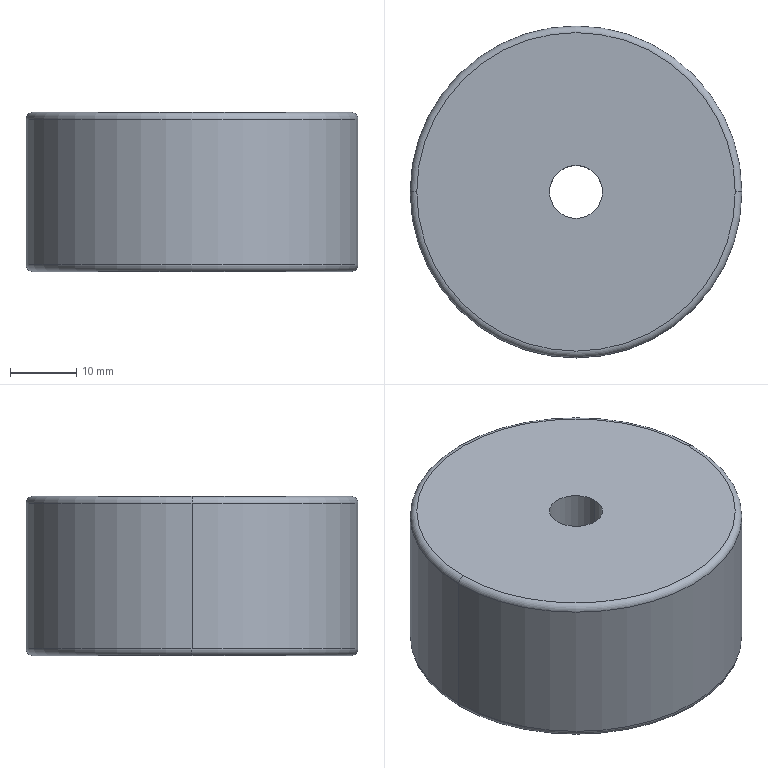Part | SolidWorks | features Extrusion 1, Fillet 1, ICE 1 | 1 solid | 10 faces | box 50 x 50 x 24 mm | volume 45851 mm3 | torus 4 | cylinder 4 | plane 2 | commonest cylinder face diameters 8 x2 50 x2
STEP:
#1=CARTESIAN_POINT('',(-25.,0.,23.));
#2=VERTEX_POINT('',#1);
#3=CARTESIAN_POINT('',(25.,0.,23.));
#4=VERTEX_POINT('',#3);
#5=CARTESIAN_POINT('',(0.,0.,23.));
#6=DIRECTION('',(0.,0.,-1.));
#7=DIRECTION('',(1.,0.,0.));
#8=AXIS2_PLACEMENT_3D('',#5,#6,#7);
#9=CIRCLE('',#8,25.);
#10=EDGE_CURVE('',#2,#4,#9,.T.);
#11=ORIENTED_EDGE('',*,*,#10,.F.);
#12=CARTESIAN_POINT('',(-24.,0.,24.));
#13=VERTEX_POINT('',#12);
#14=CARTESIAN_POINT('',(-24.,0.,23.));
#15=DIRECTION('',(0.,1.,0.));
#16=DIRECTION('',(-1.,0.,0.));
#17=AXIS2_PLACEMENT_3D('',#14,#15,#16);
#18=CIRCLE('',#17,1.);
#19=EDGE_CURVE('',#2,#13,#18,.T.);
#20=ORIENTED_EDGE('',*,*,#19,.T.);
#21=CARTESIAN_POINT('',(24.,0.,24.));
#22=VERTEX_POINT('',#21);
#23=CARTESIAN_POINT('',(0.,0.,24.));
#24=DIRECTION('',(0.,0.,1.));
#25=DIRECTION('',(1.,0.,0.));
#26=AXIS2_PLACEMENT_3D('',#23,#24,#25);
#27=CIRCLE('',#26,24.);
#28=EDGE_CURVE('',#22,#13,#27,.T.);
#29=ORIENTED_EDGE('',*,*,#28,.F.);
#30=CARTESIAN_POINT('',(24.,0.,23.));
#31=DIRECTION('',(0.,-1.,0.));
#32=DIRECTION('',(0.,0.,-1.));
#33=AXIS2_PLACEMENT_3D('',#30,#31,#32);
#34=CIRCLE('',#33,1.);
#35=EDGE_CURVE('',#4,#22,#34,.T.);
#36=ORIENTED_EDGE('',*,*,#35,.F.);
#37=EDGE_LOOP('',(#11,#20,#29,#36));
#38=FACE_OUTER_BOUND('',#37,.T.);
#39=CARTESIAN_POINT('',(0.,0.,23.));
#40=DIRECTION('',(0.,0.,1.));
#41=DIRECTION('',(1.,0.,0.));
#42=AXIS2_PLACEMENT_3D('',#39,#40,#41);
#43=TOROIDAL_SURFACE('',#42,24.,1.);
#44=ADVANCED_FACE('',(#38),#43,.T.);
#45=CARTESIAN_POINT('',(-24.,0.,0.));
#46=VERTEX_POINT('',#45);
#47=CARTESIAN_POINT('',(24.,0.,0.));
#48=VERTEX_POINT('',#47);
#49=CARTESIAN_POINT('',(0.,0.,0.));
#50=DIRECTION('',(0.,0.,-1.));
#51=DIRECTION('',(1.,0.,0.));
#52=AXIS2_PLACEMENT_3D('',#49,#50,#51);
#53=CIRCLE('',#52,24.);
#54=EDGE_CURVE('',#46,#48,#53,.T.);
#55=ORIENTED_EDGE('',*,*,#54,.F.);
#56=CARTESIAN_POINT('',(-25.,0.,1.));
#57=VERTEX_POINT('',#56);
#58=CARTESIAN_POINT('',(-24.,0.,1.));
#59=DIRECTION('',(0.,1.,0.));
#60=DIRECTION('',(-1.,0.,0.));
#61=AXIS2_PLACEMENT_3D('',#58,#59,#60);
#62=CIRCLE('',#61,1.);
#63=EDGE_CURVE('',#46,#57,#62,.T.);
#64=ORIENTED_EDGE('',*,*,#63,.T.);
#65=CARTESIAN_POINT('',(25.,0.,1.));
#66=VERTEX_POINT('',#65);
#67=CARTESIAN_POINT('',(0.,0.,1.));
#68=DIRECTION('',(0.,0.,1.));
#69=DIRECTION('',(1.,0.,0.));
#70=AXIS2_PLACEMENT_3D('',#67,#68,#69);
#71=CIRCLE('',#70,25.);
#72=EDGE_CURVE('',#66,#57,#71,.T.);
#73=ORIENTED_EDGE('',*,*,#72,.F.);
#74=CARTESIAN_POINT('',(24.,0.,1.));
#75=DIRECTION('',(0.,-1.,0.));
#76=DIRECTION('',(0.,0.,-1.));
#77=AXIS2_PLACEMENT_3D('',#74,#75,#76);
#78=CIRCLE('',#77,1.);
#79=EDGE_CURVE('',#48,#66,#78,.T.);
#80=ORIENTED_EDGE('',*,*,#79,.F.);
#81=EDGE_LOOP('',(#55,#64,#73,#80));
#82=FACE_OUTER_BOUND('',#81,.T.);
#83=CARTESIAN_POINT('',(0.,0.,1.));
#84=DIRECTION('',(0.,0.,1.));
#85=DIRECTION('',(1.,0.,0.));
#86=AXIS2_PLACEMENT_3D('',#83,#84,#85);
#87=TOROIDAL_SURFACE('',#86,24.,1.);
#88=ADVANCED_FACE('',(#82),#87,.T.);
#89=CARTESIAN_POINT('',(-4.,0.,0.));
#90=VERTEX_POINT('',#89);
#91=CARTESIAN_POINT('',(4.,0.,0.));
#92=VERTEX_POINT('',#91);
#93=CARTESIAN_POINT('',(0.,0.,0.));
#94=DIRECTION('',(0.,0.,1.));
#95=DIRECTION('',(1.,0.,0.));
#96=AXIS2_PLACEMENT_3D('',#93,#94,#95);
#97=CIRCLE('',#96,4.);
#98=EDGE_CURVE('',#90,#92,#97,.T.);
#99=ORIENTED_EDGE('',*,*,#98,.F.);
#100=CARTESIAN_POINT('',(-4.,0.,24.));
#101=VERTEX_POINT('',#100);
#102=CARTESIAN_POINT('',(-4.,0.,0.));
#103=DIRECTION('',(0.,0.,1.));
#104=VECTOR('',#103,1000.);
#105=LINE('',#102,#104);
#106=EDGE_CURVE('',#90,#101,#105,.T.);
#107=ORIENTED_EDGE('',*,*,#106,.T.);
#108=CARTESIAN_POINT('',(4.,0.,24.));
#109=VERTEX_POINT('',#108);
#110=CARTESIAN_POINT('',(0.,0.,24.));
#111=DIRECTION('',(0.,0.,1.));
#112=DIRECTION('',(1.,0.,0.));
#113=AXIS2_PLACEMENT_3D('',#110,#111,#112);
#114=CIRCLE('',#113,4.);
#115=EDGE_CURVE('',#101,#109,#114,.T.);
#116=ORIENTED_EDGE('',*,*,#115,.T.);
#117=CARTESIAN_POINT('',(4.,0.,0.));
#118=DIRECTION('',(0.,0.,1.));
#119=VECTOR('',#118,1000.);
#120=LINE('',#117,#119);
#121=EDGE_CURVE('',#92,#109,#120,.T.);
#122=ORIENTED_EDGE('',*,*,#121,.F.);
#123=EDGE_LOOP('',(#99,#107,#116,#122));
#124=FACE_OUTER_BOUND('',#123,.T.);
#125=CARTESIAN_POINT('',(0.,0.,0.));
#126=DIRECTION('',(0.,0.,1.));
#127=DIRECTION('',(1.,0.,0.));
#128=AXIS2_PLACEMENT_3D('',#125,#126,#127);
#129=CYLINDRICAL_SURFACE('',#128,4.);
#130=ADVANCED_FACE('',(#124),#129,.F.);
#131=ORIENTED_EDGE('',*,*,#10,.T.);
#132=CARTESIAN_POINT('',(25.,0.,24.));
#133=DIRECTION('',(0.,0.,-1.));
#134=VECTOR('',#133,1000.);
#135=LINE('',#132,#134);
#136=EDGE_CURVE('',#4,#66,#135,.T.);
#137=ORIENTED_EDGE('',*,*,#136,.T.);
#138=ORIENTED_EDGE('',*,*,#72,.T.);
#139=CARTESIAN_POINT('',(-25.,0.,24.));
#140=DIRECTION('',(0.,0.,-1.));
#141=VECTOR('',#140,1000.);
#142=LINE('',#139,#141);
#143=EDGE_CURVE('',#2,#57,#142,.T.);
#144=ORIENTED_EDGE('',*,*,#143,.F.);
#145=EDGE_LOOP('',(#131,#137,#138,#144));
#146=FACE_OUTER_BOUND('',#145,.T.);
#147=CARTESIAN_POINT('',(0.,0.,24.));
#148=DIRECTION('',(0.,0.,-1.));
#149=DIRECTION('',(-1.,0.,0.));
#150=AXIS2_PLACEMENT_3D('',#147,#148,#149);
#151=CYLINDRICAL_SURFACE('',#150,25.);
#152=ADVANCED_FACE('',(#146),#151,.T.);
#153=ORIENTED_EDGE('',*,*,#136,.F.);
#154=CARTESIAN_POINT('',(0.,0.,23.));
#155=DIRECTION('',(0.,0.,-1.));
#156=DIRECTION('',(1.,0.,0.));
#157=AXIS2_PLACEMENT_3D('',#154,#155,#156);
#158=CIRCLE('',#157,25.);
#159=EDGE_CURVE('',#4,#2,#158,.T.);
#160=ORIENTED_EDGE('',*,*,#159,.T.);
#161=ORIENTED_EDGE('',*,*,#143,.T.);
#162=CARTESIAN_POINT('',(0.,0.,1.));
#163=DIRECTION('',(0.,0.,1.));
#164=DIRECTION('',(1.,0.,0.));
#165=AXIS2_PLACEMENT_3D('',#162,#163,#164);
#166=CIRCLE('',#165,25.);
#167=EDGE_CURVE('',#57,#66,#166,.T.);
#168=ORIENTED_EDGE('',*,*,#167,.T.);
#169=EDGE_LOOP('',(#153,#160,#161,#168));
#170=FACE_OUTER_BOUND('',#169,.T.);
#171=CARTESIAN_POINT('',(0.,0.,24.));
#172=DIRECTION('',(0.,0.,-1.));
#173=DIRECTION('',(-1.,0.,0.));
#174=AXIS2_PLACEMENT_3D('',#171,#172,#173);
#175=CYLINDRICAL_SURFACE('',#174,25.);
#176=ADVANCED_FACE('',(#170),#175,.T.);
#177=ORIENTED_EDGE('',*,*,#28,.T.);
#178=CARTESIAN_POINT('',(0.,0.,24.));
#179=DIRECTION('',(0.,0.,1.));
#180=DIRECTION('',(1.,0.,0.));
#181=AXIS2_PLACEMENT_3D('',#178,#179,#180);
#182=CIRCLE('',#181,24.);
#183=EDGE_CURVE('',#13,#22,#182,.T.);
#184=ORIENTED_EDGE('',*,*,#183,.T.);
#185=EDGE_LOOP('',(#177,#184));
#186=FACE_OUTER_BOUND('',#185,.T.);
#187=CARTESIAN_POINT('',(0.,0.,24.));
#188=DIRECTION('',(0.,0.,1.));
#189=DIRECTION('',(1.,0.,0.));
#190=AXIS2_PLACEMENT_3D('',#187,#188,#189);
#191=CIRCLE('',#190,4.);
#192=EDGE_CURVE('',#109,#101,#191,.T.);
#193=ORIENTED_EDGE('',*,*,#192,.F.);
#194=ORIENTED_EDGE('',*,*,#115,.F.);
#195=EDGE_LOOP('',(#193,#194));
#196=FACE_BOUND('',#195,.T.);
#197=CARTESIAN_POINT('',(0.,0.,24.));
#198=DIRECTION('',(0.,0.,1.));
#199=DIRECTION('',(1.,0.,0.));
#200=AXIS2_PLACEMENT_3D('',#197,#198,#199);
#201=PLANE('',#200);
#202=ADVANCED_FACE('',(#186,#196),#201,.T.);
#203=CARTESIAN_POINT('',(0.,0.,0.));
#204=DIRECTION('',(0.,0.,-1.));
#205=DIRECTION('',(1.,0.,0.));
#206=AXIS2_PLACEMENT_3D('',#203,#204,#205);
#207=CIRCLE('',#206,24.);
#208=EDGE_CURVE('',#48,#46,#207,.T.);
#209=ORIENTED_EDGE('',*,*,#208,.T.);
#210=ORIENTED_EDGE('',*,*,#54,.T.);
#211=EDGE_LOOP('',(#209,#210));
#212=FACE_OUTER_BOUND('',#211,.T.);
#213=CARTESIAN_POINT('',(0.,0.,0.));
#214=DIRECTION('',(0.,0.,1.));
#215=DIRECTION('',(1.,0.,0.));
#216=AXIS2_PLACEMENT_3D('',#213,#214,#215);
#217=CIRCLE('',#216,4.);
#218=EDGE_CURVE('',#92,#90,#217,.T.);
#219=ORIENTED_EDGE('',*,*,#218,.T.);
#220=ORIENTED_EDGE('',*,*,#98,.T.);
#221=EDGE_LOOP('',(#219,#220));
#222=FACE_BOUND('',#221,.T.);
#223=CARTESIAN_POINT('',(0.,0.,0.));
#224=DIRECTION('',(0.,0.,1.));
#225=DIRECTION('',(1.,0.,0.));
#226=AXIS2_PLACEMENT_3D('',#223,#224,#225);
#227=PLANE('',#226);
#228=ADVANCED_FACE('',(#212,#222),#227,.F.);
#229=ORIENTED_EDGE('',*,*,#106,.F.);
#230=ORIENTED_EDGE('',*,*,#218,.F.);
#231=ORIENTED_EDGE('',*,*,#121,.T.);
#232=ORIENTED_EDGE('',*,*,#192,.T.);
#233=EDGE_LOOP('',(#229,#230,#231,#232));
#234=FACE_OUTER_BOUND('',#233,.T.);
#235=CARTESIAN_POINT('',(0.,0.,0.));
#236=DIRECTION('',(0.,0.,1.));
#237=DIRECTION('',(1.,0.,0.));
#238=AXIS2_PLACEMENT_3D('',#235,#236,#237);
#239=CYLINDRICAL_SURFACE('',#238,4.);
#240=ADVANCED_FACE('',(#234),#239,.F.);
#241=ORIENTED_EDGE('',*,*,#63,.F.);
#242=ORIENTED_EDGE('',*,*,#208,.F.);
#243=ORIENTED_EDGE('',*,*,#79,.T.);
#244=ORIENTED_EDGE('',*,*,#167,.F.);
#245=EDGE_LOOP('',(#241,#242,#243,#244));
#246=FACE_OUTER_BOUND('',#245,.T.);
#247=CARTESIAN_POINT('',(0.,0.,1.));
#248=DIRECTION('',(0.,0.,1.));
#249=DIRECTION('',(1.,0.,0.));
#250=AXIS2_PLACEMENT_3D('',#247,#248,#249);
#251=TOROIDAL_SURFACE('',#250,24.,1.);
#252=ADVANCED_FACE('',(#246),#251,.T.);
#253=ORIENTED_EDGE('',*,*,#19,.F.);
#254=ORIENTED_EDGE('',*,*,#159,.F.);
#255=ORIENTED_EDGE('',*,*,#35,.T.);
#256=ORIENTED_EDGE('',*,*,#183,.F.);
#257=EDGE_LOOP('',(#253,#254,#255,#256));
#258=FACE_OUTER_BOUND('',#257,.T.);
#259=CARTESIAN_POINT('',(0.,0.,23.));
#260=DIRECTION('',(0.,0.,1.));
#261=DIRECTION('',(1.,0.,0.));
#262=AXIS2_PLACEMENT_3D('',#259,#260,#261);
#263=TOROIDAL_SURFACE('',#262,24.,1.);
#264=ADVANCED_FACE('',(#258),#263,.T.);
#265=CLOSED_SHELL('',(#44,#88,#130,#152,#176,#202,#228,#240,#252,#264));
#266=MANIFOLD_SOLID_BREP('',#265);
#267=CARTESIAN_POINT('',(0.,0.,0.));
#268=DIRECTION('',(0.,0.,1.));
#269=DIRECTION('',(1.,0.,0.));
#270=AXIS2_PLACEMENT_3D('',#267,#268,#269);
#271=(LENGTH_UNIT()NAMED_UNIT(*)SI_UNIT(.MILLI.,.METRE.));
#272=UNCERTAINTY_MEASURE_WITH_UNIT(LENGTH_MEASURE(0.00001),#271,'','');
#273=(NAMED_UNIT(*)PLANE_ANGLE_UNIT()SI_UNIT($,.RADIAN.));
#274=(NAMED_UNIT(*)SI_UNIT($,.STERADIAN.)SOLID_ANGLE_UNIT());
#275=(GEOMETRIC_REPRESENTATION_CONTEXT(3)GLOBAL_UNCERTAINTY_ASSIGNED_CONTEXT((#272))GLOBAL_UNIT_ASSIGNED_CONTEXT((#271,#273,#274))REPRESENTATION_CONTEXT('',''));
#276=ADVANCED_BREP_SHAPE_REPRESENTATION('',(#266,#270),#275);